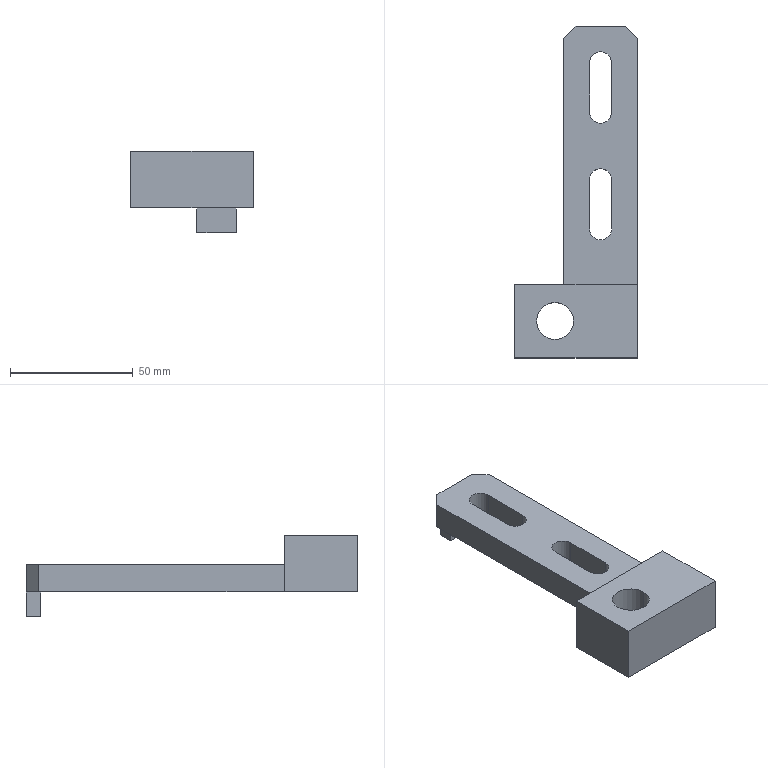Part | STEP file | Tensioner wheel bracket | 1 solid | 25 faces | box 50 x 135 x 33 mm | volume 60411 mm3 | plane 19 | cylinder 6 | commonest cylinder face diameters 9 x4 15 x2